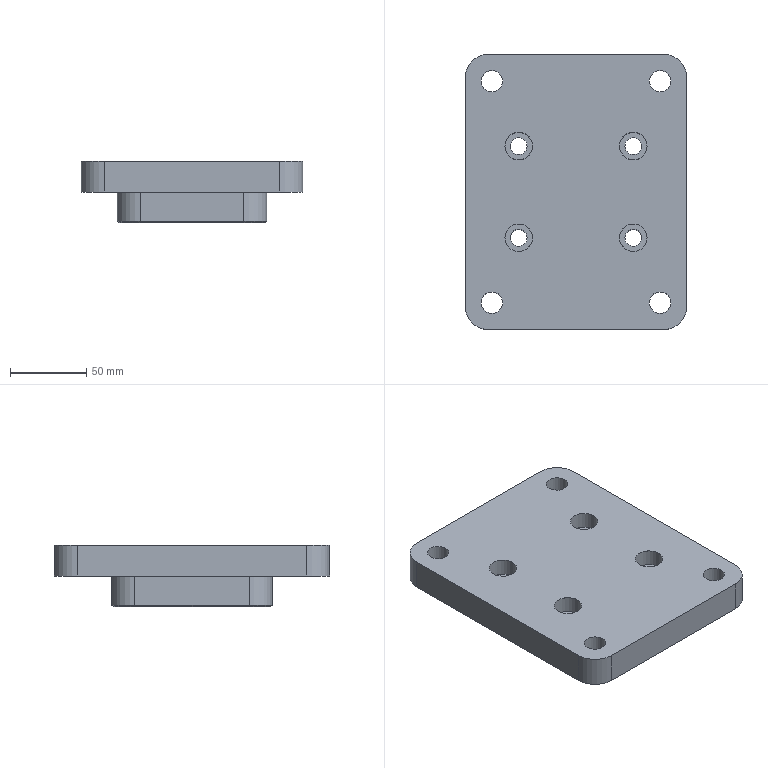NC program | NX | posted with a generic post | part box 145 x 180 x 40 mm
Lines 1 to 39 of 5818:
N10 G17 G21 G94 G90
(DRILLING , TOOL : ZXZ)
N12 T01 M6
N14 G54
N16 G17 G0 G90 X-72.5 Y-55. S5000 M3
N18 G43 Z30. H1
N20 G94 G81 G98 Z-1. F250. R3.
N22 X-30. Y-37.5
N24 X30.
N26 X72.5 Y-55.
N28 Y55.
N30 X30. Y37.5
N32 X-30.
N34 X-72.5 Y55.
N36 G80
N38 G0 X-72.5 Y55. Z30.
N40 M5
(DRILLING_COPY , TOOL : 11.0ZT)
N42 T13 M6
N44 G54
N46 G17 G0 G90 X-72.5 Y-55. S2000 M3
N48 G43 Z30. H13
N50 G94 G83 G98 Z-24.805 F200. Q2. R3.
N52 X-30. Y-37.5 Z-44.805
N54 X30.
N56 X72.5 Y-55. Z-24.805
N58 Y55.
N60 X30. Y37.5 Z-44.805
N62 X-30.
N64 X-72.5 Y55. Z-24.805
N66 G80
N68 G0 X-72.5 Y55. Z30.
N70 M5